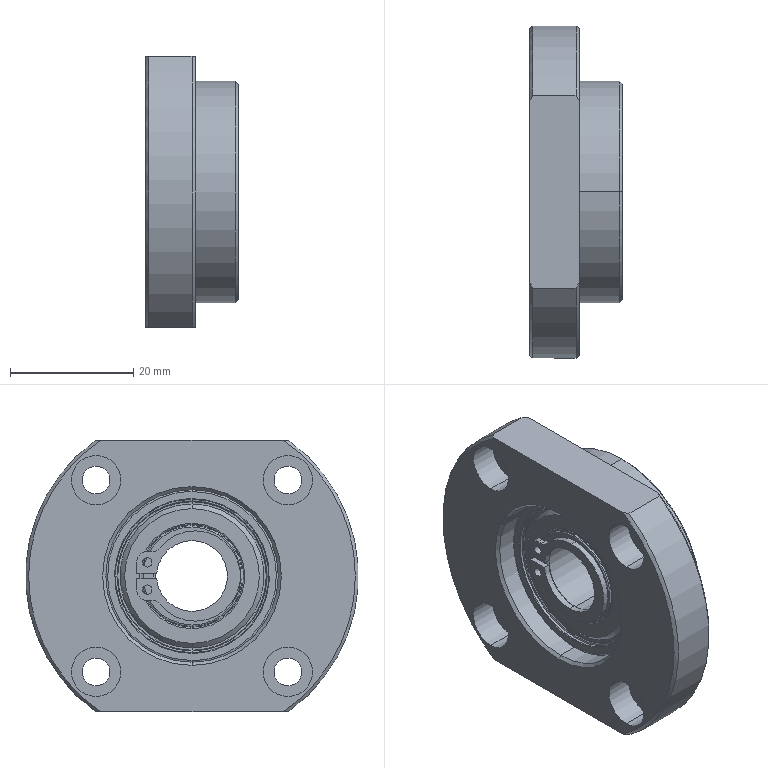Part | SolidWorks | 3 solids | 199 faces | box 15 x 54 x 44 mm | volume 16597 mm3 | cylinder 68 | spline 52 | cone 50 | plane 29 | commonest cylinder face diameters 4.5 x8 8 x8 1.5 x4 3.4 x4 15.5 x4 16.3 x4